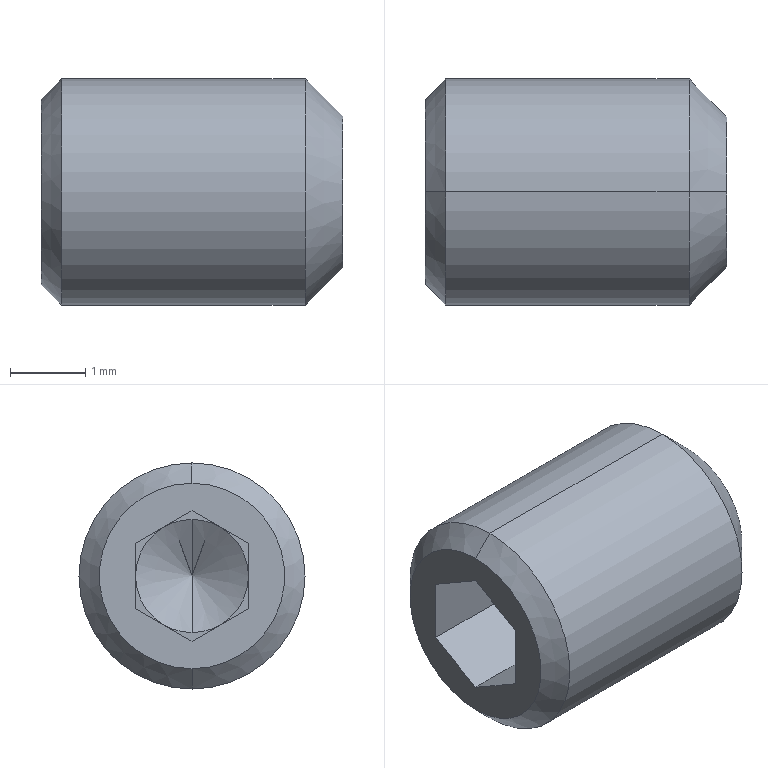Part | STEP file | hex socket set screws with flat point gb_GB_FASTENER_SCREWS_HSFP M3X4-N_1.step-36.STEP.STEP-585.STEP | 1 solid | 22 faces | box 4 x 3 x 3 mm | volume 24.31 mm3 | plane 14 | cone 6 | cylinder 2 | commonest cylinder face diameters 3 x2
STEP:
#1=CARTESIAN_POINT('',(3.5,0.,1.5));
#2=VERTEX_POINT('',#1);
#3=CARTESIAN_POINT('',(3.5,0.,-1.5));
#4=VERTEX_POINT('',#3);
#5=CARTESIAN_POINT('',(3.5,0.,0.));
#6=DIRECTION('',(-1.,0.,0.));
#7=DIRECTION('',(0.,0.,1.));
#8=AXIS2_PLACEMENT_3D('',#5,#6,#7);
#9=CIRCLE('',#8,1.5);
#10=EDGE_CURVE('',#2,#4,#9,.T.);
#11=ORIENTED_EDGE('',*,*,#10,.T.);
#12=CARTESIAN_POINT('',(0.2705,0.,-1.5));
#13=VERTEX_POINT('',#12);
#14=CARTESIAN_POINT('',(-10.745,0.,-1.5));
#15=DIRECTION('',(-1.,0.,0.));
#16=VECTOR('',#15,1000.);
#17=LINE('',#14,#16);
#18=EDGE_CURVE('',#4,#13,#17,.T.);
#19=ORIENTED_EDGE('',*,*,#18,.T.);
#20=CARTESIAN_POINT('',(0.2705,0.,1.5));
#21=VERTEX_POINT('',#20);
#22=CARTESIAN_POINT('',(0.2705,0.,0.));
#23=DIRECTION('',(1.,0.,0.));
#24=DIRECTION('',(0.,0.,1.));
#25=AXIS2_PLACEMENT_3D('',#22,#23,#24);
#26=CIRCLE('',#25,1.5);
#27=EDGE_CURVE('',#13,#21,#26,.T.);
#28=ORIENTED_EDGE('',*,*,#27,.T.);
#29=CARTESIAN_POINT('',(-10.745,0.,1.5));
#30=DIRECTION('',(-1.,0.,0.));
#31=VECTOR('',#30,1000.);
#32=LINE('',#29,#31);
#33=EDGE_CURVE('',#2,#21,#32,.T.);
#34=ORIENTED_EDGE('',*,*,#33,.F.);
#35=EDGE_LOOP('',(#11,#19,#28,#34));
#36=FACE_OUTER_BOUND('',#35,.T.);
#37=CARTESIAN_POINT('',(-10.745,0.,0.));
#38=DIRECTION('',(-1.,0.,0.));
#39=DIRECTION('',(0.,0.,1.));
#40=AXIS2_PLACEMENT_3D('',#37,#38,#39);
#41=CYLINDRICAL_SURFACE('',#40,1.5);
#42=ADVANCED_FACE('',(#36),#41,.T.);
#43=CARTESIAN_POINT('',(4.,0.,1.));
#44=VERTEX_POINT('',#43);
#45=CARTESIAN_POINT('',(4.,0.,-1.));
#46=VERTEX_POINT('',#45);
#47=CARTESIAN_POINT('',(4.,0.,0.));
#48=DIRECTION('',(-1.,0.,0.));
#49=DIRECTION('',(0.,0.,1.));
#50=AXIS2_PLACEMENT_3D('',#47,#48,#49);
#51=CIRCLE('',#50,1.);
#52=EDGE_CURVE('',#44,#46,#51,.T.);
#53=ORIENTED_EDGE('',*,*,#52,.T.);
#54=CARTESIAN_POINT('',(3.5,0.,-1.5));
#55=DIRECTION('',(-0.7071,0.,-0.7071));
#56=VECTOR('',#55,1000.);
#57=LINE('',#54,#56);
#58=EDGE_CURVE('',#46,#4,#57,.T.);
#59=ORIENTED_EDGE('',*,*,#58,.T.);
#60=ORIENTED_EDGE('',*,*,#10,.F.);
#61=CARTESIAN_POINT('',(3.5,0.,1.5));
#62=DIRECTION('',(-0.7071,0.,0.7071));
#63=VECTOR('',#62,1000.);
#64=LINE('',#61,#63);
#65=EDGE_CURVE('',#44,#2,#64,.T.);
#66=ORIENTED_EDGE('',*,*,#65,.F.);
#67=EDGE_LOOP('',(#53,#59,#60,#66));
#68=FACE_OUTER_BOUND('',#67,.T.);
#69=CARTESIAN_POINT('',(3.5,0.,0.));
#70=DIRECTION('',(-1.,0.,0.));
#71=DIRECTION('',(0.,0.,1.));
#72=AXIS2_PLACEMENT_3D('',#69,#70,#71);
#73=CONICAL_SURFACE('',#72,1.5,0.7854);
#74=ADVANCED_FACE('',(#68),#73,.T.);
#75=CARTESIAN_POINT('',(0.,0.,-1.23));
#76=VERTEX_POINT('',#75);
#77=CARTESIAN_POINT('',(0.,0.,1.23));
#78=VERTEX_POINT('',#77);
#79=CARTESIAN_POINT('',(0.,0.,0.));
#80=DIRECTION('',(1.,0.,0.));
#81=DIRECTION('',(0.,0.,-1.));
#82=AXIS2_PLACEMENT_3D('',#79,#80,#81);
#83=CIRCLE('',#82,1.23);
#84=EDGE_CURVE('',#76,#78,#83,.T.);
#85=ORIENTED_EDGE('',*,*,#84,.T.);
#86=CARTESIAN_POINT('',(0.2705,0.,1.5));
#87=DIRECTION('',(0.7071,0.,0.7071));
#88=VECTOR('',#87,1000.);
#89=LINE('',#86,#88);
#90=EDGE_CURVE('',#78,#21,#89,.T.);
#91=ORIENTED_EDGE('',*,*,#90,.T.);
#92=ORIENTED_EDGE('',*,*,#27,.F.);
#93=CARTESIAN_POINT('',(0.2705,0.,-1.5));
#94=DIRECTION('',(0.7071,0.,-0.7071));
#95=VECTOR('',#94,1000.);
#96=LINE('',#93,#95);
#97=EDGE_CURVE('',#76,#13,#96,.T.);
#98=ORIENTED_EDGE('',*,*,#97,.F.);
#99=EDGE_LOOP('',(#85,#91,#92,#98));
#100=FACE_OUTER_BOUND('',#99,.T.);
#101=CARTESIAN_POINT('',(0.2705,0.,0.));
#102=DIRECTION('',(1.,0.,0.));
#103=DIRECTION('',(0.,0.,-1.));
#104=AXIS2_PLACEMENT_3D('',#101,#102,#103);
#105=CONICAL_SURFACE('',#104,1.5,0.7854);
#106=ADVANCED_FACE('',(#100),#105,.T.);
#107=CARTESIAN_POINT('',(1.633,0.,0.));
#108=VERTEX_POINT('',#107);
#109=CARTESIAN_POINT('',(1.2,0.,0.75));
#110=VERTEX_POINT('',#109);
#111=CARTESIAN_POINT('',(1.2,0.,0.75));
#112=DIRECTION('',(-0.5,0.,0.866));
#113=VECTOR('',#112,1000.);
#114=LINE('',#111,#113);
#115=EDGE_CURVE('',#108,#110,#114,.T.);
#116=ORIENTED_EDGE('',*,*,#115,.F.);
#117=CARTESIAN_POINT('',(1.2,0.,-0.75));
#118=VERTEX_POINT('',#117);
#119=CARTESIAN_POINT('',(1.2,0.,-0.75));
#120=DIRECTION('',(-0.5,0.,-0.866));
#121=VECTOR('',#120,1000.);
#122=LINE('',#119,#121);
#123=EDGE_CURVE('',#108,#118,#122,.T.);
#124=ORIENTED_EDGE('',*,*,#123,.T.);
#125=CARTESIAN_POINT('',(1.2,-0.375,-0.6495));
#126=VERTEX_POINT('',#125);
#127=CARTESIAN_POINT('',(1.2,0.,0.));
#128=DIRECTION('',(1.,0.,0.));
#129=DIRECTION('',(0.,0.,1.));
#130=AXIS2_PLACEMENT_3D('',#127,#128,#129);
#131=CIRCLE('',#130,0.75);
#132=EDGE_CURVE('',#126,#118,#131,.T.);
#133=ORIENTED_EDGE('',*,*,#132,.F.);
#134=CARTESIAN_POINT('',(1.2,-0.75,0.));
#135=VERTEX_POINT('',#134);
#136=CARTESIAN_POINT('',(1.2,0.,0.));
#137=DIRECTION('',(1.,0.,0.));
#138=DIRECTION('',(0.,0.,1.));
#139=AXIS2_PLACEMENT_3D('',#136,#137,#138);
#140=CIRCLE('',#139,0.75);
#141=EDGE_CURVE('',#135,#126,#140,.T.);
#142=ORIENTED_EDGE('',*,*,#141,.F.);
#143=CARTESIAN_POINT('',(1.2,-0.375,0.6495));
#144=VERTEX_POINT('',#143);
#145=CARTESIAN_POINT('',(1.2,0.,0.));
#146=DIRECTION('',(1.,0.,0.));
#147=DIRECTION('',(0.,0.,1.));
#148=AXIS2_PLACEMENT_3D('',#145,#146,#147);
#149=CIRCLE('',#148,0.75);
#150=EDGE_CURVE('',#144,#135,#149,.T.);
#151=ORIENTED_EDGE('',*,*,#150,.F.);
#152=CARTESIAN_POINT('',(1.2,0.,0.));
#153=DIRECTION('',(1.,0.,0.));
#154=DIRECTION('',(0.,0.,1.));
#155=AXIS2_PLACEMENT_3D('',#152,#153,#154);
#156=CIRCLE('',#155,0.75);
#157=EDGE_CURVE('',#110,#144,#156,.T.);
#158=ORIENTED_EDGE('',*,*,#157,.F.);
#159=EDGE_LOOP('',(#116,#124,#133,#142,#151,#158));
#160=FACE_OUTER_BOUND('',#159,.T.);
#161=CARTESIAN_POINT('',(1.2,0.,0.));
#162=DIRECTION('',(-1.,0.,0.));
#163=DIRECTION('',(0.,0.,1.));
#164=AXIS2_PLACEMENT_3D('',#161,#162,#163);
#165=CONICAL_SURFACE('',#164,0.75,1.047);
#166=ADVANCED_FACE('',(#160),#165,.F.);
#167=ORIENTED_EDGE('',*,*,#18,.F.);
#168=CARTESIAN_POINT('',(3.5,0.,0.));
#169=DIRECTION('',(-1.,0.,0.));
#170=DIRECTION('',(0.,0.,1.));
#171=AXIS2_PLACEMENT_3D('',#168,#169,#170);
#172=CIRCLE('',#171,1.5);
#173=EDGE_CURVE('',#4,#2,#172,.T.);
#174=ORIENTED_EDGE('',*,*,#173,.T.);
#175=ORIENTED_EDGE('',*,*,#33,.T.);
#176=CARTESIAN_POINT('',(0.2705,0.,0.));
#177=DIRECTION('',(1.,0.,0.));
#178=DIRECTION('',(0.,0.,1.));
#179=AXIS2_PLACEMENT_3D('',#176,#177,#178);
#180=CIRCLE('',#179,1.5);
#181=EDGE_CURVE('',#21,#13,#180,.T.);
#182=ORIENTED_EDGE('',*,*,#181,.T.);
#183=EDGE_LOOP('',(#167,#174,#175,#182));
#184=FACE_OUTER_BOUND('',#183,.T.);
#185=CARTESIAN_POINT('',(-10.745,0.,0.));
#186=DIRECTION('',(-1.,0.,0.));
#187=DIRECTION('',(0.,0.,1.));
#188=AXIS2_PLACEMENT_3D('',#185,#186,#187);
#189=CYLINDRICAL_SURFACE('',#188,1.5);
#190=ADVANCED_FACE('',(#184),#189,.T.);
#191=ORIENTED_EDGE('',*,*,#58,.F.);
#192=CARTESIAN_POINT('',(4.,0.,0.));
#193=DIRECTION('',(-1.,0.,0.));
#194=DIRECTION('',(0.,0.,1.));
#195=AXIS2_PLACEMENT_3D('',#192,#193,#194);
#196=CIRCLE('',#195,1.);
#197=EDGE_CURVE('',#46,#44,#196,.T.);
#198=ORIENTED_EDGE('',*,*,#197,.T.);
#199=ORIENTED_EDGE('',*,*,#65,.T.);
#200=ORIENTED_EDGE('',*,*,#173,.F.);
#201=EDGE_LOOP('',(#191,#198,#199,#200));
#202=FACE_OUTER_BOUND('',#201,.T.);
#203=CARTESIAN_POINT('',(3.5,0.,0.));
#204=DIRECTION('',(-1.,0.,0.));
#205=DIRECTION('',(0.,0.,1.));
#206=AXIS2_PLACEMENT_3D('',#203,#204,#205);
#207=CONICAL_SURFACE('',#206,1.5,0.7854);
#208=ADVANCED_FACE('',(#202),#207,.T.);
#209=ORIENTED_EDGE('',*,*,#90,.F.);
#210=CARTESIAN_POINT('',(0.,0.,0.));
#211=DIRECTION('',(1.,0.,0.));
#212=DIRECTION('',(0.,0.,-1.));
#213=AXIS2_PLACEMENT_3D('',#210,#211,#212);
#214=CIRCLE('',#213,1.23);
#215=EDGE_CURVE('',#78,#76,#214,.T.);
#216=ORIENTED_EDGE('',*,*,#215,.T.);
#217=ORIENTED_EDGE('',*,*,#97,.T.);
#218=ORIENTED_EDGE('',*,*,#181,.F.);
#219=EDGE_LOOP('',(#209,#216,#217,#218));
#220=FACE_OUTER_BOUND('',#219,.T.);
#221=CARTESIAN_POINT('',(0.2705,0.,0.));
#222=DIRECTION('',(1.,0.,0.));
#223=DIRECTION('',(0.,0.,-1.));
#224=AXIS2_PLACEMENT_3D('',#221,#222,#223);
#225=CONICAL_SURFACE('',#224,1.5,0.7854);
#226=ADVANCED_FACE('',(#220),#225,.T.);
#227=ORIENTED_EDGE('',*,*,#52,.F.);
#228=ORIENTED_EDGE('',*,*,#197,.F.);
#229=EDGE_LOOP('',(#227,#228));
#230=FACE_OUTER_BOUND('',#229,.T.);
#231=CARTESIAN_POINT('',(4.,0.,0.));
#232=DIRECTION('',(-1.,0.,0.));
#233=DIRECTION('',(0.,0.,1.));
#234=AXIS2_PLACEMENT_3D('',#231,#232,#233);
#235=PLANE('',#234);
#236=ADVANCED_FACE('',(#230),#235,.F.);
#237=CARTESIAN_POINT('',(0.,-0.75,-0.433));
#238=VERTEX_POINT('',#237);
#239=CARTESIAN_POINT('',(0.,-0.75,0.433));
#240=VERTEX_POINT('',#239);
#241=CARTESIAN_POINT('',(0.,-0.75,0.));
#242=DIRECTION('',(0.,0.,1.));
#243=VECTOR('',#242,1000.);
#244=LINE('',#241,#243);
#245=EDGE_CURVE('',#238,#240,#244,.T.);
#246=ORIENTED_EDGE('',*,*,#245,.F.);
#247=CARTESIAN_POINT('',(0.,0.,-0.866));
#248=VERTEX_POINT('',#247);
#249=CARTESIAN_POINT('',(0.,0.,-0.866));
#250=DIRECTION('',(0.,-0.866,0.5));
#251=VECTOR('',#250,1000.);
#252=LINE('',#249,#251);
#253=EDGE_CURVE('',#248,#238,#252,.T.);
#254=ORIENTED_EDGE('',*,*,#253,.F.);
#255=CARTESIAN_POINT('',(0.,0.75,-0.433));
#256=VERTEX_POINT('',#255);
#257=CARTESIAN_POINT('',(0.,0.75,-0.433));
#258=DIRECTION('',(0.,-0.866,-0.5));
#259=VECTOR('',#258,1000.);
#260=LINE('',#257,#259);
#261=EDGE_CURVE('',#256,#248,#260,.T.);
#262=ORIENTED_EDGE('',*,*,#261,.F.);
#263=CARTESIAN_POINT('',(0.,0.75,0.433));
#264=VERTEX_POINT('',#263);
#265=CARTESIAN_POINT('',(0.,0.75,0.));
#266=DIRECTION('',(0.,0.,-1.));
#267=VECTOR('',#266,1000.);
#268=LINE('',#265,#267);
#269=EDGE_CURVE('',#264,#256,#268,.T.);
#270=ORIENTED_EDGE('',*,*,#269,.F.);
#271=CARTESIAN_POINT('',(0.,0.,0.866));
#272=VERTEX_POINT('',#271);
#273=CARTESIAN_POINT('',(0.,0.,0.866));
#274=DIRECTION('',(0.,0.866,-0.5));
#275=VECTOR('',#274,1000.);
#276=LINE('',#273,#275);
#277=EDGE_CURVE('',#272,#264,#276,.T.);
#278=ORIENTED_EDGE('',*,*,#277,.F.);
#279=CARTESIAN_POINT('',(0.,-0.75,0.433));
#280=DIRECTION('',(0.,0.866,0.5));
#281=VECTOR('',#280,1000.);
#282=LINE('',#279,#281);
#283=EDGE_CURVE('',#240,#272,#282,.T.);
#284=ORIENTED_EDGE('',*,*,#283,.F.);
#285=EDGE_LOOP('',(#246,#254,#262,#270,#278,#284));
#286=FACE_BOUND('',#285,.T.);
#287=ORIENTED_EDGE('',*,*,#84,.F.);
#288=ORIENTED_EDGE('',*,*,#215,.F.);
#289=EDGE_LOOP('',(#287,#288));
#290=FACE_OUTER_BOUND('',#289,.T.);
#291=CARTESIAN_POINT('',(0.,1.229,0.));
#292=DIRECTION('',(1.,0.,0.));
#293=DIRECTION('',(0.,1.,0.));
#294=AXIS2_PLACEMENT_3D('',#291,#292,#293);
#295=PLANE('',#294);
#296=ADVANCED_FACE('',(#286,#290),#295,.F.);
#297=CARTESIAN_POINT('',(1.2,0.,0.866));
#298=VERTEX_POINT('',#297);
#299=CARTESIAN_POINT('',(1.2,-0.75,0.433));
#300=DIRECTION('',(0.,0.866,0.5));
#301=VECTOR('',#300,1000.);
#302=LINE('',#299,#301);
#303=EDGE_CURVE('',#144,#298,#302,.T.);
#304=ORIENTED_EDGE('',*,*,#303,.F.);
#305=CARTESIAN_POINT('',(1.2,-0.75,0.433));
#306=VERTEX_POINT('',#305);
#307=CARTESIAN_POINT('',(1.2,-0.75,0.433));
#308=DIRECTION('',(0.,0.866,0.5));
#309=VECTOR('',#308,1000.);
#310=LINE('',#307,#309);
#311=EDGE_CURVE('',#306,#144,#310,.T.);
#312=ORIENTED_EDGE('',*,*,#311,.F.);
#313=CARTESIAN_POINT('',(1.2,-0.75,0.433));
#314=DIRECTION('',(1.,0.,0.));
#315=VECTOR('',#314,1000.);
#316=LINE('',#313,#315);
#317=EDGE_CURVE('',#240,#306,#316,.T.);
#318=ORIENTED_EDGE('',*,*,#317,.F.);
#319=ORIENTED_EDGE('',*,*,#283,.T.);
#320=CARTESIAN_POINT('',(1.2,0.,0.866));
#321=DIRECTION('',(-1.,0.,0.));
#322=VECTOR('',#321,1000.);
#323=LINE('',#320,#322);
#324=EDGE_CURVE('',#298,#272,#323,.T.);
#325=ORIENTED_EDGE('',*,*,#324,.F.);
#326=EDGE_LOOP('',(#304,#312,#318,#319,#325));
#327=FACE_OUTER_BOUND('',#326,.T.);
#328=CARTESIAN_POINT('',(1.2,-0.75,0.433));
#329=DIRECTION('',(0.,-0.5,0.866));
#330=DIRECTION('',(-1.,0.,0.));
#331=AXIS2_PLACEMENT_3D('',#328,#329,#330);
#332=PLANE('',#331);
#333=ADVANCED_FACE('',(#327),#332,.F.);
#334=CARTESIAN_POINT('',(1.2,-0.75,-0.433));
#335=DIRECTION('',(0.,0.,1.));
#336=VECTOR('',#335,1000.);
#337=LINE('',#334,#336);
#338=EDGE_CURVE('',#135,#306,#337,.T.);
#339=ORIENTED_EDGE('',*,*,#338,.F.);
#340=CARTESIAN_POINT('',(1.2,-0.75,-0.433));
#341=VERTEX_POINT('',#340);
#342=CARTESIAN_POINT('',(1.2,-0.75,-0.433));
#343=DIRECTION('',(0.,0.,1.));
#344=VECTOR('',#343,1000.);
#345=LINE('',#342,#344);
#346=EDGE_CURVE('',#341,#135,#345,.T.);
#347=ORIENTED_EDGE('',*,*,#346,.F.);
#348=CARTESIAN_POINT('',(1.2,-0.75,-0.433));
#349=DIRECTION('',(1.,0.,0.));
#350=VECTOR('',#349,1000.);
#351=LINE('',#348,#350);
#352=EDGE_CURVE('',#238,#341,#351,.T.);
#353=ORIENTED_EDGE('',*,*,#352,.F.);
#354=ORIENTED_EDGE('',*,*,#245,.T.);
#355=ORIENTED_EDGE('',*,*,#317,.T.);
#356=EDGE_LOOP('',(#339,#347,#353,#354,#355));
#357=FACE_OUTER_BOUND('',#356,.T.);
#358=CARTESIAN_POINT('',(1.2,-0.75,-0.433));
#359=DIRECTION('',(0.,-1.,0.));
#360=DIRECTION('',(0.,0.,-1.));
#361=AXIS2_PLACEMENT_3D('',#358,#359,#360);
#362=PLANE('',#361);
#363=ADVANCED_FACE('',(#357),#362,.F.);
#364=CARTESIAN_POINT('',(1.2,0.,-0.866));
#365=DIRECTION('',(0.,-0.866,0.5));
#366=VECTOR('',#365,1000.);
#367=LINE('',#364,#366);
#368=EDGE_CURVE('',#126,#341,#367,.T.);
#369=ORIENTED_EDGE('',*,*,#368,.F.);
#370=CARTESIAN_POINT('',(1.2,0.,-0.866));
#371=VERTEX_POINT('',#370);
#372=CARTESIAN_POINT('',(1.2,0.,-0.866));
#373=DIRECTION('',(0.,-0.866,0.5));
#374=VECTOR('',#373,1000.);
#375=LINE('',#372,#374);
#376=EDGE_CURVE('',#371,#126,#375,.T.);
#377=ORIENTED_EDGE('',*,*,#376,.F.);
#378=CARTESIAN_POINT('',(1.2,0.,-0.866));
#379=DIRECTION('',(1.,0.,0.));
#380=VECTOR('',#379,1000.);
#381=LINE('',#378,#380);
#382=EDGE_CURVE('',#248,#371,#381,.T.);
#383=ORIENTED_EDGE('',*,*,#382,.F.);
#384=ORIENTED_EDGE('',*,*,#253,.T.);
#385=ORIENTED_EDGE('',*,*,#352,.T.);
#386=EDGE_LOOP('',(#369,#377,#383,#384,#385));
#387=FACE_OUTER_BOUND('',#386,.T.);
#388=CARTESIAN_POINT('',(1.2,0.,-0.866));
#389=DIRECTION('',(0.,-0.5,-0.866));
#390=DIRECTION('',(0.,-0.866,0.5));
#391=AXIS2_PLACEMENT_3D('',#388,#389,#390);
#392=PLANE('',#391);
#393=ADVANCED_FACE('',(#387),#392,.F.);
#394=CARTESIAN_POINT('',(1.2,0.375,-0.6495));
#395=VERTEX_POINT('',#394);
#396=CARTESIAN_POINT('',(1.2,0.75,-0.433));
#397=DIRECTION('',(0.,-0.866,-0.5));
#398=VECTOR('',#397,1000.);
#399=LINE('',#396,#398);
#400=EDGE_CURVE('',#395,#371,#399,.T.);
#401=ORIENTED_EDGE('',*,*,#400,.F.);
#402=CARTESIAN_POINT('',(1.2,0.75,-0.433));
#403=VERTEX_POINT('',#402);
#404=CARTESIAN_POINT('',(1.2,0.75,-0.433));
#405=DIRECTION('',(0.,-0.866,-0.5));
#406=VECTOR('',#405,1000.);
#407=LINE('',#404,#406);
#408=EDGE_CURVE('',#403,#395,#407,.T.);
#409=ORIENTED_EDGE('',*,*,#408,.F.);
#410=CARTESIAN_POINT('',(1.2,0.75,-0.433));
#411=DIRECTION('',(1.,0.,0.));
#412=VECTOR('',#411,1000.);
#413=LINE('',#410,#412);
#414=EDGE_CURVE('',#256,#403,#413,.T.);
#415=ORIENTED_EDGE('',*,*,#414,.F.);
#416=ORIENTED_EDGE('',*,*,#261,.T.);
#417=ORIENTED_EDGE('',*,*,#382,.T.);
#418=EDGE_LOOP('',(#401,#409,#415,#416,#417));
#419=FACE_OUTER_BOUND('',#418,.T.);
#420=CARTESIAN_POINT('',(1.2,0.75,-0.433));
#421=DIRECTION('',(0.,0.5,-0.866));
#422=DIRECTION('',(-1.,0.,0.));
#423=AXIS2_PLACEMENT_3D('',#420,#421,#422);
#424=PLANE('',#423);
#425=ADVANCED_FACE('',(#419),#424,.F.);
#426=CARTESIAN_POINT('',(1.2,0.75,0.));
#427=VERTEX_POINT('',#426);
#428=CARTESIAN_POINT('',(1.2,0.75,0.433));
#429=DIRECTION('',(0.,0.,-1.));
#430=VECTOR('',#429,1000.);
#431=LINE('',#428,#430);
#432=EDGE_CURVE('',#427,#403,#431,.T.);
#433=ORIENTED_EDGE('',*,*,#432,.F.);
#434=CARTESIAN_POINT('',(1.2,0.75,0.433));
#435=VERTEX_POINT('',#434);
#436=CARTESIAN_POINT('',(1.2,0.75,0.433));
#437=DIRECTION('',(0.,0.,-1.));
#438=VECTOR('',#437,1000.);
#439=LINE('',#436,#438);
#440=EDGE_CURVE('',#435,#427,#439,.T.);
#441=ORIENTED_EDGE('',*,*,#440,.F.);
#442=CARTESIAN_POINT('',(1.2,0.75,0.433));
#443=DIRECTION('',(1.,0.,0.));
#444=VECTOR('',#443,1000.);
#445=LINE('',#442,#444);
#446=EDGE_CURVE('',#264,#435,#445,.T.);
#447=ORIENTED_EDGE('',*,*,#446,.F.);
#448=ORIENTED_EDGE('',*,*,#269,.T.);
#449=ORIENTED_EDGE('',*,*,#414,.T.);
#450=EDGE_LOOP('',(#433,#441,#447,#448,#449));
#451=FACE_OUTER_BOUND('',#450,.T.);
#452=CARTESIAN_POINT('',(1.2,0.75,0.433));
#453=DIRECTION('',(0.,1.,0.));
#454=DIRECTION('',(1.,0.,0.));
#455=AXIS2_PLACEMENT_3D('',#452,#453,#454);
#456=PLANE('',#455);
#457=ADVANCED_FACE('',(#451),#456,.F.);
#458=CARTESIAN_POINT('',(1.2,0.375,0.6495));
#459=VERTEX_POINT('',#458);
#460=CARTESIAN_POINT('',(1.2,0.,0.866));
#461=DIRECTION('',(0.,0.866,-0.5));
#462=VECTOR('',#461,1000.);
#463=LINE('',#460,#462);
#464=EDGE_CURVE('',#459,#435,#463,.T.);
#465=ORIENTED_EDGE('',*,*,#464,.F.);
#466=CARTESIAN_POINT('',(1.2,0.,0.866));
#467=DIRECTION('',(0.,0.866,-0.5));
#468=VECTOR('',#467,1000.);
#469=LINE('',#466,#468);
#470=EDGE_CURVE('',#298,#459,#469,.T.);
#471=ORIENTED_EDGE('',*,*,#470,.F.);
#472=ORIENTED_EDGE('',*,*,#324,.T.);
#473=ORIENTED_EDGE('',*,*,#277,.T.);
#474=ORIENTED_EDGE('',*,*,#446,.T.);
#475=EDGE_LOOP('',(#465,#471,#472,#473,#474));
#476=FACE_OUTER_BOUND('',#475,.T.);
#477=CARTESIAN_POINT('',(1.2,0.,0.866));
#478=DIRECTION('',(0.,0.5,0.866));
#479=DIRECTION('',(1.,0.,0.));
#480=AXIS2_PLACEMENT_3D('',#477,#478,#479);
#481=PLANE('',#480);
#482=ADVANCED_FACE('',(#476),#481,.F.);
#483=CARTESIAN_POINT('',(1.2,0.,0.));
#484=DIRECTION('',(1.,0.,0.));
#485=DIRECTION('',(0.,0.,1.));
#486=AXIS2_PLACEMENT_3D('',#483,#484,#485);
#487=CIRCLE('',#486,0.75);
#488=EDGE_CURVE('',#459,#110,#487,.T.);
#489=ORIENTED_EDGE('',*,*,#488,.T.);
#490=ORIENTED_EDGE('',*,*,#157,.T.);
#491=ORIENTED_EDGE('',*,*,#303,.T.);
#492=ORIENTED_EDGE('',*,*,#470,.T.);
#493=EDGE_LOOP('',(#489,#490,#491,#492));
#494=FACE_OUTER_BOUND('',#493,.T.);
#495=CARTESIAN_POINT('',(1.2,0.,0.866));
#496=DIRECTION('',(-1.,0.,0.));
#497=DIRECTION('',(0.,0.,1.));
#498=AXIS2_PLACEMENT_3D('',#495,#496,#497);
#499=PLANE('',#498);
#500=ADVANCED_FACE('',(#494),#499,.T.);
#501=ORIENTED_EDGE('',*,*,#311,.T.);
#502=ORIENTED_EDGE('',*,*,#150,.T.);
#503=ORIENTED_EDGE('',*,*,#338,.T.);
#504=EDGE_LOOP('',(#501,#502,#503));
#505=FACE_OUTER_BOUND('',#504,.T.);
#506=CARTESIAN_POINT('',(1.2,0.,0.866));
#507=DIRECTION('',(-1.,0.,0.));
#508=DIRECTION('',(0.,0.,1.));
#509=AXIS2_PLACEMENT_3D('',#506,#507,#508);
#510=PLANE('',#509);
#511=ADVANCED_FACE('',(#505),#510,.T.);
#512=ORIENTED_EDGE('',*,*,#346,.T.);
#513=ORIENTED_EDGE('',*,*,#141,.T.);
#514=ORIENTED_EDGE('',*,*,#368,.T.);
#515=EDGE_LOOP('',(#512,#513,#514));
#516=FACE_OUTER_BOUND('',#515,.T.);
#517=CARTESIAN_POINT('',(1.2,0.,0.866));
#518=DIRECTION('',(-1.,0.,0.));
#519=DIRECTION('',(0.,0.,1.));
#520=AXIS2_PLACEMENT_3D('',#517,#518,#519);
#521=PLANE('',#520);
#522=ADVANCED_FACE('',(#516),#521,.T.);
#523=ORIENTED_EDGE('',*,*,#132,.T.);
#524=CARTESIAN_POINT('',(1.2,0.,0.));
#525=DIRECTION('',(1.,0.,0.));
#526=DIRECTION('',(0.,0.,1.));
#527=AXIS2_PLACEMENT_3D('',#524,#525,#526);
#528=CIRCLE('',#527,0.75);
#529=EDGE_CURVE('',#118,#395,#528,.T.);
#530=ORIENTED_EDGE('',*,*,#529,.T.);
#531=ORIENTED_EDGE('',*,*,#400,.T.);
#532=ORIENTED_EDGE('',*,*,#376,.T.);
#533=EDGE_LOOP('',(#523,#530,#531,#532));
#534=FACE_OUTER_BOUND('',#533,.T.);
#535=CARTESIAN_POINT('',(1.2,0.,0.866));
#536=DIRECTION('',(-1.,0.,0.));
#537=DIRECTION('',(0.,0.,1.));
#538=AXIS2_PLACEMENT_3D('',#535,#536,#537);
#539=PLANE('',#538);
#540=ADVANCED_FACE('',(#534),#539,.T.);
#541=ORIENTED_EDGE('',*,*,#408,.T.);
#542=CARTESIAN_POINT('',(1.2,0.,0.));
#543=DIRECTION('',(1.,0.,0.));
#544=DIRECTION('',(0.,0.,1.));
#545=AXIS2_PLACEMENT_3D('',#542,#543,#544);
#546=CIRCLE('',#545,0.75);
#547=EDGE_CURVE('',#395,#427,#546,.T.);
#548=ORIENTED_EDGE('',*,*,#547,.T.);
#549=ORIENTED_EDGE('',*,*,#432,.T.);
#550=EDGE_LOOP('',(#541,#548,#549));
#551=FACE_OUTER_BOUND('',#550,.T.);
#552=CARTESIAN_POINT('',(1.2,0.,0.866));
#553=DIRECTION('',(-1.,0.,0.));
#554=DIRECTION('',(0.,0.,1.));
#555=AXIS2_PLACEMENT_3D('',#552,#553,#554);
#556=PLANE('',#555);
#557=ADVANCED_FACE('',(#551),#556,.T.);
#558=ORIENTED_EDGE('',*,*,#440,.T.);
#559=CARTESIAN_POINT('',(1.2,0.,0.));
#560=DIRECTION('',(1.,0.,0.));
#561=DIRECTION('',(0.,0.,1.));
#562=AXIS2_PLACEMENT_3D('',#559,#560,#561);
#563=CIRCLE('',#562,0.75);
#564=EDGE_CURVE('',#427,#459,#563,.T.);
#565=ORIENTED_EDGE('',*,*,#564,.T.);
#566=ORIENTED_EDGE('',*,*,#464,.T.);
#567=EDGE_LOOP('',(#558,#565,#566));
#568=FACE_OUTER_BOUND('',#567,.T.);
#569=CARTESIAN_POINT('',(1.2,0.,0.866));
#570=DIRECTION('',(-1.,0.,0.));
#571=DIRECTION('',(0.,0.,1.));
#572=AXIS2_PLACEMENT_3D('',#569,#570,#571);
#573=PLANE('',#572);
#574=ADVANCED_FACE('',(#568),#573,.T.);
#575=ORIENTED_EDGE('',*,*,#123,.F.);
#576=ORIENTED_EDGE('',*,*,#115,.T.);
#577=ORIENTED_EDGE('',*,*,#488,.F.);
#578=ORIENTED_EDGE('',*,*,#564,.F.);
#579=ORIENTED_EDGE('',*,*,#547,.F.);
#580=ORIENTED_EDGE('',*,*,#529,.F.);
#581=EDGE_LOOP('',(#575,#576,#577,#578,#579,#580));
#582=FACE_OUTER_BOUND('',#581,.T.);
#583=CARTESIAN_POINT('',(1.2,0.,0.));
#584=DIRECTION('',(-1.,0.,0.));
#585=DIRECTION('',(0.,0.,1.));
#586=AXIS2_PLACEMENT_3D('',#583,#584,#585);
#587=CONICAL_SURFACE('',#586,0.75,1.047);
#588=ADVANCED_FACE('',(#582),#587,.F.);
#589=CLOSED_SHELL('',(#42,#74,#106,#166,#190,#208,#226,#236,#296,#333,#363,#393,#425,#457,#482,#500,#511,#522,#540,#557,#574,#588));
#590=MANIFOLD_SOLID_BREP('',#589);
#591=CARTESIAN_POINT('',(0.,0.,0.));
#592=DIRECTION('',(0.,0.,1.));
#593=DIRECTION('',(1.,0.,0.));
#594=AXIS2_PLACEMENT_3D('',#591,#592,#593);
#595=(LENGTH_UNIT()NAMED_UNIT(*)SI_UNIT(.MILLI.,.METRE.));
#596=UNCERTAINTY_MEASURE_WITH_UNIT(LENGTH_MEASURE(0.00001),#595,'','');
#597=(NAMED_UNIT(*)PLANE_ANGLE_UNIT()SI_UNIT($,.RADIAN.));
#598=(NAMED_UNIT(*)SI_UNIT($,.STERADIAN.)SOLID_ANGLE_UNIT());
#599=(GEOMETRIC_REPRESENTATION_CONTEXT(3)GLOBAL_UNCERTAINTY_ASSIGNED_CONTEXT((#596))GLOBAL_UNIT_ASSIGNED_CONTEXT((#595,#597,#598))REPRESENTATION_CONTEXT('',''));
#600=ADVANCED_BREP_SHAPE_REPRESENTATION('',(#590,#594),#599);